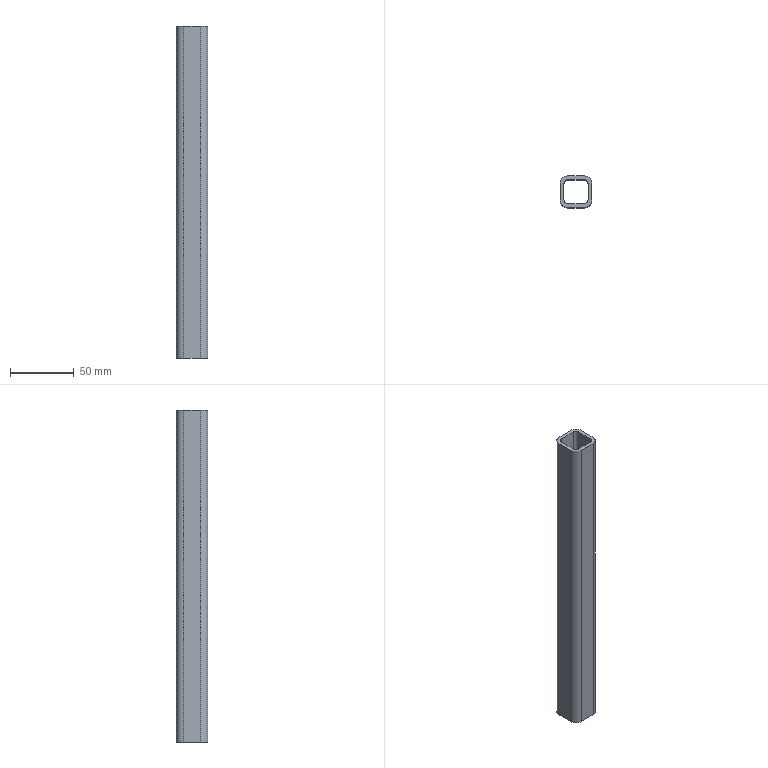Part | STEP file | ISO 10799-2 25x25x3 1784906820679 | 1 solid | 18 faces | box 25 x 25 x 261 mm | volume 62855 mm3 | plane 10 | cylinder 8 | commonest cylinder face diameters 6 x4 12 x4
STEP:
#1=CARTESIAN_POINT('',(-6.5,-9.5,286.));
#2=VERTEX_POINT('',#1);
#3=CARTESIAN_POINT('',(6.5,-9.5,286.));
#4=VERTEX_POINT('',#3);
#5=CARTESIAN_POINT('',(3.25,-9.5,286.));
#6=DIRECTION('',(1.,0.,0.));
#7=VECTOR('',#6,10.);
#8=LINE('',#5,#7);
#9=EDGE_CURVE('',#2,#4,#8,.T.);
#10=ORIENTED_EDGE('',*,*,#9,.T.);
#11=CARTESIAN_POINT('',(6.5,-9.5,25.));
#12=VERTEX_POINT('',#11);
#13=CARTESIAN_POINT('',(6.5,-9.5,0.));
#14=DIRECTION('',(0.,0.,1.));
#15=VECTOR('',#14,10.);
#16=LINE('',#13,#15);
#17=EDGE_CURVE('',#12,#4,#16,.T.);
#18=ORIENTED_EDGE('',*,*,#17,.F.);
#19=CARTESIAN_POINT('',(-6.5,-9.5,25.));
#20=VERTEX_POINT('',#19);
#21=CARTESIAN_POINT('',(3.25,-9.5,25.));
#22=DIRECTION('',(1.,0.,0.));
#23=VECTOR('',#22,10.);
#24=LINE('',#21,#23);
#25=EDGE_CURVE('',#20,#12,#24,.T.);
#26=ORIENTED_EDGE('',*,*,#25,.F.);
#27=CARTESIAN_POINT('',(-6.5,-9.5,0.));
#28=DIRECTION('',(0.,0.,1.));
#29=VECTOR('',#28,10.);
#30=LINE('',#27,#29);
#31=EDGE_CURVE('',#20,#2,#30,.T.);
#32=ORIENTED_EDGE('',*,*,#31,.T.);
#33=EDGE_LOOP('',(#10,#18,#26,#32));
#34=FACE_OUTER_BOUND('',#33,.T.);
#35=CARTESIAN_POINT('',(6.5,-9.5,0.));
#36=DIRECTION('',(0.,-1.,0.));
#37=DIRECTION('',(0.,0.,-1.));
#38=AXIS2_PLACEMENT_3D('',#35,#36,#37);
#39=PLANE('',#38);
#40=ADVANCED_FACE('',(#34),#39,.F.);
#41=CARTESIAN_POINT('',(9.5,-6.5,286.));
#42=VERTEX_POINT('',#41);
#43=CARTESIAN_POINT('',(6.5,-6.5,286.));
#44=DIRECTION('',(0.,0.,1.));
#45=DIRECTION('',(0.,1.,0.));
#46=AXIS2_PLACEMENT_3D('',#43,#44,#45);
#47=CIRCLE('',#46,3.);
#48=EDGE_CURVE('',#4,#42,#47,.T.);
#49=ORIENTED_EDGE('',*,*,#48,.T.);
#50=CARTESIAN_POINT('',(9.5,-6.5,25.));
#51=VERTEX_POINT('',#50);
#52=CARTESIAN_POINT('',(9.5,-6.5,0.));
#53=DIRECTION('',(0.,0.,1.));
#54=VECTOR('',#53,10.);
#55=LINE('',#52,#54);
#56=EDGE_CURVE('',#51,#42,#55,.T.);
#57=ORIENTED_EDGE('',*,*,#56,.F.);
#58=CARTESIAN_POINT('',(6.5,-6.5,25.));
#59=DIRECTION('',(0.,0.,1.));
#60=DIRECTION('',(0.,1.,0.));
#61=AXIS2_PLACEMENT_3D('',#58,#59,#60);
#62=CIRCLE('',#61,3.);
#63=EDGE_CURVE('',#12,#51,#62,.T.);
#64=ORIENTED_EDGE('',*,*,#63,.F.);
#65=ORIENTED_EDGE('',*,*,#17,.T.);
#66=EDGE_LOOP('',(#49,#57,#64,#65));
#67=FACE_OUTER_BOUND('',#66,.T.);
#68=CARTESIAN_POINT('',(6.5,-6.5,0.));
#69=DIRECTION('',(0.,0.,1.));
#70=DIRECTION('',(0.,1.,0.));
#71=AXIS2_PLACEMENT_3D('',#68,#69,#70);
#72=CYLINDRICAL_SURFACE('',#71,3.);
#73=ADVANCED_FACE('',(#67),#72,.F.);
#74=CARTESIAN_POINT('',(9.5,6.5,286.));
#75=VERTEX_POINT('',#74);
#76=CARTESIAN_POINT('',(9.5,3.25,286.));
#77=DIRECTION('',(0.,1.,0.));
#78=VECTOR('',#77,10.);
#79=LINE('',#76,#78);
#80=EDGE_CURVE('',#42,#75,#79,.T.);
#81=ORIENTED_EDGE('',*,*,#80,.T.);
#82=CARTESIAN_POINT('',(9.5,6.5,25.));
#83=VERTEX_POINT('',#82);
#84=CARTESIAN_POINT('',(9.5,6.5,0.));
#85=DIRECTION('',(0.,0.,1.));
#86=VECTOR('',#85,10.);
#87=LINE('',#84,#86);
#88=EDGE_CURVE('',#83,#75,#87,.T.);
#89=ORIENTED_EDGE('',*,*,#88,.F.);
#90=CARTESIAN_POINT('',(9.5,3.25,25.));
#91=DIRECTION('',(0.,1.,0.));
#92=VECTOR('',#91,10.);
#93=LINE('',#90,#92);
#94=EDGE_CURVE('',#51,#83,#93,.T.);
#95=ORIENTED_EDGE('',*,*,#94,.F.);
#96=ORIENTED_EDGE('',*,*,#56,.T.);
#97=EDGE_LOOP('',(#81,#89,#95,#96));
#98=FACE_OUTER_BOUND('',#97,.T.);
#99=CARTESIAN_POINT('',(9.5,6.5,0.));
#100=DIRECTION('',(1.,0.,0.));
#101=DIRECTION('',(0.,0.,-1.));
#102=AXIS2_PLACEMENT_3D('',#99,#100,#101);
#103=PLANE('',#102);
#104=ADVANCED_FACE('',(#98),#103,.F.);
#105=CARTESIAN_POINT('',(6.5,9.5,286.));
#106=VERTEX_POINT('',#105);
#107=CARTESIAN_POINT('',(6.5,6.5,286.));
#108=DIRECTION('',(0.,0.,1.));
#109=DIRECTION('',(-1.,0.,0.));
#110=AXIS2_PLACEMENT_3D('',#107,#108,#109);
#111=CIRCLE('',#110,3.);
#112=EDGE_CURVE('',#75,#106,#111,.T.);
#113=ORIENTED_EDGE('',*,*,#112,.T.);
#114=CARTESIAN_POINT('',(6.5,9.5,25.));
#115=VERTEX_POINT('',#114);
#116=CARTESIAN_POINT('',(6.5,9.5,0.));
#117=DIRECTION('',(0.,0.,1.));
#118=VECTOR('',#117,10.);
#119=LINE('',#116,#118);
#120=EDGE_CURVE('',#115,#106,#119,.T.);
#121=ORIENTED_EDGE('',*,*,#120,.F.);
#122=CARTESIAN_POINT('',(6.5,6.5,25.));
#123=DIRECTION('',(0.,0.,1.));
#124=DIRECTION('',(-1.,0.,0.));
#125=AXIS2_PLACEMENT_3D('',#122,#123,#124);
#126=CIRCLE('',#125,3.);
#127=EDGE_CURVE('',#83,#115,#126,.T.);
#128=ORIENTED_EDGE('',*,*,#127,.F.);
#129=ORIENTED_EDGE('',*,*,#88,.T.);
#130=EDGE_LOOP('',(#113,#121,#128,#129));
#131=FACE_OUTER_BOUND('',#130,.T.);
#132=CARTESIAN_POINT('',(6.5,6.5,0.));
#133=DIRECTION('',(0.,0.,1.));
#134=DIRECTION('',(-1.,0.,0.));
#135=AXIS2_PLACEMENT_3D('',#132,#133,#134);
#136=CYLINDRICAL_SURFACE('',#135,3.);
#137=ADVANCED_FACE('',(#131),#136,.F.);
#138=CARTESIAN_POINT('',(12.5,6.5,286.));
#139=VERTEX_POINT('',#138);
#140=CARTESIAN_POINT('',(12.5,-6.5,286.));
#141=VERTEX_POINT('',#140);
#142=CARTESIAN_POINT('',(12.5,3.25,286.));
#143=DIRECTION('',(0.,-1.,0.));
#144=VECTOR('',#143,10.);
#145=LINE('',#142,#144);
#146=EDGE_CURVE('',#139,#141,#145,.T.);
#147=ORIENTED_EDGE('',*,*,#146,.T.);
#148=CARTESIAN_POINT('',(12.5,-6.5,25.));
#149=VERTEX_POINT('',#148);
#150=CARTESIAN_POINT('',(12.5,-6.5,0.));
#151=DIRECTION('',(0.,0.,1.));
#152=VECTOR('',#151,10.);
#153=LINE('',#150,#152);
#154=EDGE_CURVE('',#149,#141,#153,.T.);
#155=ORIENTED_EDGE('',*,*,#154,.F.);
#156=CARTESIAN_POINT('',(12.5,6.5,25.));
#157=VERTEX_POINT('',#156);
#158=CARTESIAN_POINT('',(12.5,3.25,25.));
#159=DIRECTION('',(0.,-1.,0.));
#160=VECTOR('',#159,10.);
#161=LINE('',#158,#160);
#162=EDGE_CURVE('',#157,#149,#161,.T.);
#163=ORIENTED_EDGE('',*,*,#162,.F.);
#164=CARTESIAN_POINT('',(12.5,6.5,0.));
#165=DIRECTION('',(0.,0.,1.));
#166=VECTOR('',#165,10.);
#167=LINE('',#164,#166);
#168=EDGE_CURVE('',#157,#139,#167,.T.);
#169=ORIENTED_EDGE('',*,*,#168,.T.);
#170=EDGE_LOOP('',(#147,#155,#163,#169));
#171=FACE_OUTER_BOUND('',#170,.T.);
#172=CARTESIAN_POINT('',(12.5,6.5,0.));
#173=DIRECTION('',(1.,0.,0.));
#174=DIRECTION('',(0.,0.,-1.));
#175=AXIS2_PLACEMENT_3D('',#172,#173,#174);
#176=PLANE('',#175);
#177=ADVANCED_FACE('',(#171),#176,.T.);
#178=CARTESIAN_POINT('',(6.5,-12.5,286.));
#179=VERTEX_POINT('',#178);
#180=CARTESIAN_POINT('',(6.5,-6.5,286.));
#181=DIRECTION('',(0.,0.,-1.));
#182=DIRECTION('',(0.,1.,0.));
#183=AXIS2_PLACEMENT_3D('',#180,#181,#182);
#184=CIRCLE('',#183,6.);
#185=EDGE_CURVE('',#141,#179,#184,.T.);
#186=ORIENTED_EDGE('',*,*,#185,.T.);
#187=CARTESIAN_POINT('',(6.5,-12.5,25.));
#188=VERTEX_POINT('',#187);
#189=CARTESIAN_POINT('',(6.5,-12.5,0.));
#190=DIRECTION('',(0.,0.,1.));
#191=VECTOR('',#190,10.);
#192=LINE('',#189,#191);
#193=EDGE_CURVE('',#188,#179,#192,.T.);
#194=ORIENTED_EDGE('',*,*,#193,.F.);
#195=CARTESIAN_POINT('',(6.5,-6.5,25.));
#196=DIRECTION('',(0.,0.,-1.));
#197=DIRECTION('',(0.,1.,0.));
#198=AXIS2_PLACEMENT_3D('',#195,#196,#197);
#199=CIRCLE('',#198,6.);
#200=EDGE_CURVE('',#149,#188,#199,.T.);
#201=ORIENTED_EDGE('',*,*,#200,.F.);
#202=ORIENTED_EDGE('',*,*,#154,.T.);
#203=EDGE_LOOP('',(#186,#194,#201,#202));
#204=FACE_OUTER_BOUND('',#203,.T.);
#205=CARTESIAN_POINT('',(6.5,-6.5,0.));
#206=DIRECTION('',(0.,0.,1.));
#207=DIRECTION('',(0.,1.,0.));
#208=AXIS2_PLACEMENT_3D('',#205,#206,#207);
#209=CYLINDRICAL_SURFACE('',#208,6.);
#210=ADVANCED_FACE('',(#204),#209,.T.);
#211=CARTESIAN_POINT('',(-6.5,-12.5,286.));
#212=VERTEX_POINT('',#211);
#213=CARTESIAN_POINT('',(3.25,-12.5,286.));
#214=DIRECTION('',(-1.,0.,0.));
#215=VECTOR('',#214,10.);
#216=LINE('',#213,#215);
#217=EDGE_CURVE('',#179,#212,#216,.T.);
#218=ORIENTED_EDGE('',*,*,#217,.T.);
#219=CARTESIAN_POINT('',(-6.5,-12.5,25.));
#220=VERTEX_POINT('',#219);
#221=CARTESIAN_POINT('',(-6.5,-12.5,0.));
#222=DIRECTION('',(0.,0.,1.));
#223=VECTOR('',#222,10.);
#224=LINE('',#221,#223);
#225=EDGE_CURVE('',#220,#212,#224,.T.);
#226=ORIENTED_EDGE('',*,*,#225,.F.);
#227=CARTESIAN_POINT('',(3.25,-12.5,25.));
#228=DIRECTION('',(-1.,0.,0.));
#229=VECTOR('',#228,10.);
#230=LINE('',#227,#229);
#231=EDGE_CURVE('',#188,#220,#230,.T.);
#232=ORIENTED_EDGE('',*,*,#231,.F.);
#233=ORIENTED_EDGE('',*,*,#193,.T.);
#234=EDGE_LOOP('',(#218,#226,#232,#233));
#235=FACE_OUTER_BOUND('',#234,.T.);
#236=CARTESIAN_POINT('',(6.5,-12.5,0.));
#237=DIRECTION('',(0.,-1.,0.));
#238=DIRECTION('',(0.,0.,-1.));
#239=AXIS2_PLACEMENT_3D('',#236,#237,#238);
#240=PLANE('',#239);
#241=ADVANCED_FACE('',(#235),#240,.T.);
#242=CARTESIAN_POINT('',(-12.5,-6.5,286.));
#243=VERTEX_POINT('',#242);
#244=CARTESIAN_POINT('',(-6.5,-6.5,286.));
#245=DIRECTION('',(0.,0.,-1.));
#246=DIRECTION('',(1.,0.,0.));
#247=AXIS2_PLACEMENT_3D('',#244,#245,#246);
#248=CIRCLE('',#247,6.);
#249=EDGE_CURVE('',#212,#243,#248,.T.);
#250=ORIENTED_EDGE('',*,*,#249,.T.);
#251=CARTESIAN_POINT('',(-12.5,-6.5,25.));
#252=VERTEX_POINT('',#251);
#253=CARTESIAN_POINT('',(-12.5,-6.5,0.));
#254=DIRECTION('',(0.,0.,1.));
#255=VECTOR('',#254,10.);
#256=LINE('',#253,#255);
#257=EDGE_CURVE('',#252,#243,#256,.T.);
#258=ORIENTED_EDGE('',*,*,#257,.F.);
#259=CARTESIAN_POINT('',(-6.5,-6.5,25.));
#260=DIRECTION('',(0.,0.,-1.));
#261=DIRECTION('',(1.,0.,0.));
#262=AXIS2_PLACEMENT_3D('',#259,#260,#261);
#263=CIRCLE('',#262,6.);
#264=EDGE_CURVE('',#220,#252,#263,.T.);
#265=ORIENTED_EDGE('',*,*,#264,.F.);
#266=ORIENTED_EDGE('',*,*,#225,.T.);
#267=EDGE_LOOP('',(#250,#258,#265,#266));
#268=FACE_OUTER_BOUND('',#267,.T.);
#269=CARTESIAN_POINT('',(-6.5,-6.5,0.));
#270=DIRECTION('',(0.,0.,1.));
#271=DIRECTION('',(1.,0.,0.));
#272=AXIS2_PLACEMENT_3D('',#269,#270,#271);
#273=CYLINDRICAL_SURFACE('',#272,6.);
#274=ADVANCED_FACE('',(#268),#273,.T.);
#275=CARTESIAN_POINT('',(-6.5,9.5,286.));
#276=VERTEX_POINT('',#275);
#277=CARTESIAN_POINT('',(-3.25,9.5,286.));
#278=DIRECTION('',(-1.,0.,0.));
#279=VECTOR('',#278,10.);
#280=LINE('',#277,#279);
#281=EDGE_CURVE('',#106,#276,#280,.T.);
#282=ORIENTED_EDGE('',*,*,#281,.T.);
#283=CARTESIAN_POINT('',(-6.5,9.5,25.));
#284=VERTEX_POINT('',#283);
#285=CARTESIAN_POINT('',(-6.5,9.5,0.));
#286=DIRECTION('',(0.,0.,1.));
#287=VECTOR('',#286,10.);
#288=LINE('',#285,#287);
#289=EDGE_CURVE('',#284,#276,#288,.T.);
#290=ORIENTED_EDGE('',*,*,#289,.F.);
#291=CARTESIAN_POINT('',(-3.25,9.5,25.));
#292=DIRECTION('',(-1.,0.,0.));
#293=VECTOR('',#292,10.);
#294=LINE('',#291,#293);
#295=EDGE_CURVE('',#115,#284,#294,.T.);
#296=ORIENTED_EDGE('',*,*,#295,.F.);
#297=ORIENTED_EDGE('',*,*,#120,.T.);
#298=EDGE_LOOP('',(#282,#290,#296,#297));
#299=FACE_OUTER_BOUND('',#298,.T.);
#300=CARTESIAN_POINT('',(-6.5,9.5,0.));
#301=DIRECTION('',(0.,1.,0.));
#302=DIRECTION('',(0.,0.,1.));
#303=AXIS2_PLACEMENT_3D('',#300,#301,#302);
#304=PLANE('',#303);
#305=ADVANCED_FACE('',(#299),#304,.F.);
#306=CARTESIAN_POINT('',(-9.5,-6.5,286.));
#307=VERTEX_POINT('',#306);
#308=CARTESIAN_POINT('',(-6.5,-6.5,286.));
#309=DIRECTION('',(0.,0.,1.));
#310=DIRECTION('',(1.,0.,0.));
#311=AXIS2_PLACEMENT_3D('',#308,#309,#310);
#312=CIRCLE('',#311,3.);
#313=EDGE_CURVE('',#307,#2,#312,.T.);
#314=ORIENTED_EDGE('',*,*,#313,.T.);
#315=ORIENTED_EDGE('',*,*,#31,.F.);
#316=CARTESIAN_POINT('',(-9.5,-6.5,25.));
#317=VERTEX_POINT('',#316);
#318=CARTESIAN_POINT('',(-6.5,-6.5,25.));
#319=DIRECTION('',(0.,0.,1.));
#320=DIRECTION('',(1.,0.,0.));
#321=AXIS2_PLACEMENT_3D('',#318,#319,#320);
#322=CIRCLE('',#321,3.);
#323=EDGE_CURVE('',#317,#20,#322,.T.);
#324=ORIENTED_EDGE('',*,*,#323,.F.);
#325=CARTESIAN_POINT('',(-9.5,-6.5,0.));
#326=DIRECTION('',(0.,0.,1.));
#327=VECTOR('',#326,10.);
#328=LINE('',#325,#327);
#329=EDGE_CURVE('',#317,#307,#328,.T.);
#330=ORIENTED_EDGE('',*,*,#329,.T.);
#331=EDGE_LOOP('',(#314,#315,#324,#330));
#332=FACE_OUTER_BOUND('',#331,.T.);
#333=CARTESIAN_POINT('',(-6.5,-6.5,0.));
#334=DIRECTION('',(0.,0.,1.));
#335=DIRECTION('',(1.,0.,0.));
#336=AXIS2_PLACEMENT_3D('',#333,#334,#335);
#337=CYLINDRICAL_SURFACE('',#336,3.);
#338=ADVANCED_FACE('',(#332),#337,.F.);
#339=CARTESIAN_POINT('',(-9.5,6.5,286.));
#340=VERTEX_POINT('',#339);
#341=CARTESIAN_POINT('',(-9.5,-3.25,286.));
#342=DIRECTION('',(0.,-1.,0.));
#343=VECTOR('',#342,10.);
#344=LINE('',#341,#343);
#345=EDGE_CURVE('',#340,#307,#344,.T.);
#346=ORIENTED_EDGE('',*,*,#345,.T.);
#347=ORIENTED_EDGE('',*,*,#329,.F.);
#348=CARTESIAN_POINT('',(-9.5,6.5,25.));
#349=VERTEX_POINT('',#348);
#350=CARTESIAN_POINT('',(-9.5,-3.25,25.));
#351=DIRECTION('',(0.,-1.,0.));
#352=VECTOR('',#351,10.);
#353=LINE('',#350,#352);
#354=EDGE_CURVE('',#349,#317,#353,.T.);
#355=ORIENTED_EDGE('',*,*,#354,.F.);
#356=CARTESIAN_POINT('',(-9.5,6.5,0.));
#357=DIRECTION('',(0.,0.,1.));
#358=VECTOR('',#357,10.);
#359=LINE('',#356,#358);
#360=EDGE_CURVE('',#349,#340,#359,.T.);
#361=ORIENTED_EDGE('',*,*,#360,.T.);
#362=EDGE_LOOP('',(#346,#347,#355,#361));
#363=FACE_OUTER_BOUND('',#362,.T.);
#364=CARTESIAN_POINT('',(-9.5,-6.5,0.));
#365=DIRECTION('',(-1.,0.,0.));
#366=DIRECTION('',(0.,0.,1.));
#367=AXIS2_PLACEMENT_3D('',#364,#365,#366);
#368=PLANE('',#367);
#369=ADVANCED_FACE('',(#363),#368,.F.);
#370=CARTESIAN_POINT('',(-6.5,6.5,286.));
#371=DIRECTION('',(0.,0.,1.));
#372=DIRECTION('',(0.,-1.,0.));
#373=AXIS2_PLACEMENT_3D('',#370,#371,#372);
#374=CIRCLE('',#373,3.);
#375=EDGE_CURVE('',#276,#340,#374,.T.);
#376=ORIENTED_EDGE('',*,*,#375,.T.);
#377=ORIENTED_EDGE('',*,*,#360,.F.);
#378=CARTESIAN_POINT('',(-6.5,6.5,25.));
#379=DIRECTION('',(0.,0.,1.));
#380=DIRECTION('',(0.,-1.,0.));
#381=AXIS2_PLACEMENT_3D('',#378,#379,#380);
#382=CIRCLE('',#381,3.);
#383=EDGE_CURVE('',#284,#349,#382,.T.);
#384=ORIENTED_EDGE('',*,*,#383,.F.);
#385=ORIENTED_EDGE('',*,*,#289,.T.);
#386=EDGE_LOOP('',(#376,#377,#384,#385));
#387=FACE_OUTER_BOUND('',#386,.T.);
#388=CARTESIAN_POINT('',(-6.5,6.5,0.));
#389=DIRECTION('',(0.,0.,1.));
#390=DIRECTION('',(0.,-1.,0.));
#391=AXIS2_PLACEMENT_3D('',#388,#389,#390);
#392=CYLINDRICAL_SURFACE('',#391,3.);
#393=ADVANCED_FACE('',(#387),#392,.F.);
#394=CARTESIAN_POINT('',(-12.5,6.5,286.));
#395=VERTEX_POINT('',#394);
#396=CARTESIAN_POINT('',(-12.5,-3.25,286.));
#397=DIRECTION('',(0.,1.,0.));
#398=VECTOR('',#397,10.);
#399=LINE('',#396,#398);
#400=EDGE_CURVE('',#243,#395,#399,.T.);
#401=ORIENTED_EDGE('',*,*,#400,.T.);
#402=CARTESIAN_POINT('',(-12.5,6.5,25.));
#403=VERTEX_POINT('',#402);
#404=CARTESIAN_POINT('',(-12.5,6.5,0.));
#405=DIRECTION('',(0.,0.,1.));
#406=VECTOR('',#405,10.);
#407=LINE('',#404,#406);
#408=EDGE_CURVE('',#403,#395,#407,.T.);
#409=ORIENTED_EDGE('',*,*,#408,.F.);
#410=CARTESIAN_POINT('',(-12.5,-3.25,25.));
#411=DIRECTION('',(0.,1.,0.));
#412=VECTOR('',#411,10.);
#413=LINE('',#410,#412);
#414=EDGE_CURVE('',#252,#403,#413,.T.);
#415=ORIENTED_EDGE('',*,*,#414,.F.);
#416=ORIENTED_EDGE('',*,*,#257,.T.);
#417=EDGE_LOOP('',(#401,#409,#415,#416));
#418=FACE_OUTER_BOUND('',#417,.T.);
#419=CARTESIAN_POINT('',(-12.5,-6.5,0.));
#420=DIRECTION('',(-1.,0.,0.));
#421=DIRECTION('',(0.,0.,1.));
#422=AXIS2_PLACEMENT_3D('',#419,#420,#421);
#423=PLANE('',#422);
#424=ADVANCED_FACE('',(#418),#423,.T.);
#425=CARTESIAN_POINT('',(-6.5,12.5,286.));
#426=VERTEX_POINT('',#425);
#427=CARTESIAN_POINT('',(-6.5,6.5,286.));
#428=DIRECTION('',(0.,0.,-1.));
#429=DIRECTION('',(0.,-1.,0.));
#430=AXIS2_PLACEMENT_3D('',#427,#428,#429);
#431=CIRCLE('',#430,6.);
#432=EDGE_CURVE('',#395,#426,#431,.T.);
#433=ORIENTED_EDGE('',*,*,#432,.T.);
#434=CARTESIAN_POINT('',(-6.5,12.5,25.));
#435=VERTEX_POINT('',#434);
#436=CARTESIAN_POINT('',(-6.5,12.5,0.));
#437=DIRECTION('',(0.,0.,1.));
#438=VECTOR('',#437,10.);
#439=LINE('',#436,#438);
#440=EDGE_CURVE('',#435,#426,#439,.T.);
#441=ORIENTED_EDGE('',*,*,#440,.F.);
#442=CARTESIAN_POINT('',(-6.5,6.5,25.));
#443=DIRECTION('',(0.,0.,-1.));
#444=DIRECTION('',(0.,-1.,0.));
#445=AXIS2_PLACEMENT_3D('',#442,#443,#444);
#446=CIRCLE('',#445,6.);
#447=EDGE_CURVE('',#403,#435,#446,.T.);
#448=ORIENTED_EDGE('',*,*,#447,.F.);
#449=ORIENTED_EDGE('',*,*,#408,.T.);
#450=EDGE_LOOP('',(#433,#441,#448,#449));
#451=FACE_OUTER_BOUND('',#450,.T.);
#452=CARTESIAN_POINT('',(-6.5,6.5,0.));
#453=DIRECTION('',(0.,0.,1.));
#454=DIRECTION('',(0.,-1.,0.));
#455=AXIS2_PLACEMENT_3D('',#452,#453,#454);
#456=CYLINDRICAL_SURFACE('',#455,6.);
#457=ADVANCED_FACE('',(#451),#456,.T.);
#458=CARTESIAN_POINT('',(6.5,12.5,286.));
#459=VERTEX_POINT('',#458);
#460=CARTESIAN_POINT('',(-3.25,12.5,286.));
#461=DIRECTION('',(1.,0.,0.));
#462=VECTOR('',#461,10.);
#463=LINE('',#460,#462);
#464=EDGE_CURVE('',#426,#459,#463,.T.);
#465=ORIENTED_EDGE('',*,*,#464,.T.);
#466=CARTESIAN_POINT('',(6.5,12.5,25.));
#467=VERTEX_POINT('',#466);
#468=CARTESIAN_POINT('',(6.5,12.5,0.));
#469=DIRECTION('',(0.,0.,1.));
#470=VECTOR('',#469,10.);
#471=LINE('',#468,#470);
#472=EDGE_CURVE('',#467,#459,#471,.T.);
#473=ORIENTED_EDGE('',*,*,#472,.F.);
#474=CARTESIAN_POINT('',(-3.25,12.5,25.));
#475=DIRECTION('',(1.,0.,0.));
#476=VECTOR('',#475,10.);
#477=LINE('',#474,#476);
#478=EDGE_CURVE('',#435,#467,#477,.T.);
#479=ORIENTED_EDGE('',*,*,#478,.F.);
#480=ORIENTED_EDGE('',*,*,#440,.T.);
#481=EDGE_LOOP('',(#465,#473,#479,#480));
#482=FACE_OUTER_BOUND('',#481,.T.);
#483=CARTESIAN_POINT('',(-6.5,12.5,0.));
#484=DIRECTION('',(0.,1.,0.));
#485=DIRECTION('',(0.,0.,1.));
#486=AXIS2_PLACEMENT_3D('',#483,#484,#485);
#487=PLANE('',#486);
#488=ADVANCED_FACE('',(#482),#487,.T.);
#489=CARTESIAN_POINT('',(6.5,6.5,286.));
#490=DIRECTION('',(0.,0.,-1.));
#491=DIRECTION('',(-1.,0.,0.));
#492=AXIS2_PLACEMENT_3D('',#489,#490,#491);
#493=CIRCLE('',#492,6.);
#494=EDGE_CURVE('',#459,#139,#493,.T.);
#495=ORIENTED_EDGE('',*,*,#494,.T.);
#496=ORIENTED_EDGE('',*,*,#168,.F.);
#497=CARTESIAN_POINT('',(6.5,6.5,25.));
#498=DIRECTION('',(0.,0.,-1.));
#499=DIRECTION('',(-1.,0.,0.));
#500=AXIS2_PLACEMENT_3D('',#497,#498,#499);
#501=CIRCLE('',#500,6.);
#502=EDGE_CURVE('',#467,#157,#501,.T.);
#503=ORIENTED_EDGE('',*,*,#502,.F.);
#504=ORIENTED_EDGE('',*,*,#472,.T.);
#505=EDGE_LOOP('',(#495,#496,#503,#504));
#506=FACE_OUTER_BOUND('',#505,.T.);
#507=CARTESIAN_POINT('',(6.5,6.5,0.));
#508=DIRECTION('',(0.,0.,1.));
#509=DIRECTION('',(-1.,0.,0.));
#510=AXIS2_PLACEMENT_3D('',#507,#508,#509);
#511=CYLINDRICAL_SURFACE('',#510,6.);
#512=ADVANCED_FACE('',(#506),#511,.T.);
#513=ORIENTED_EDGE('',*,*,#414,.T.);
#514=ORIENTED_EDGE('',*,*,#447,.T.);
#515=ORIENTED_EDGE('',*,*,#478,.T.);
#516=ORIENTED_EDGE('',*,*,#502,.T.);
#517=ORIENTED_EDGE('',*,*,#162,.T.);
#518=ORIENTED_EDGE('',*,*,#200,.T.);
#519=ORIENTED_EDGE('',*,*,#231,.T.);
#520=ORIENTED_EDGE('',*,*,#264,.T.);
#521=EDGE_LOOP('',(#513,#514,#515,#516,#517,#518,#519,#520));
#522=FACE_OUTER_BOUND('',#521,.T.);
#523=ORIENTED_EDGE('',*,*,#295,.T.);
#524=ORIENTED_EDGE('',*,*,#383,.T.);
#525=ORIENTED_EDGE('',*,*,#354,.T.);
#526=ORIENTED_EDGE('',*,*,#323,.T.);
#527=ORIENTED_EDGE('',*,*,#25,.T.);
#528=ORIENTED_EDGE('',*,*,#63,.T.);
#529=ORIENTED_EDGE('',*,*,#94,.T.);
#530=ORIENTED_EDGE('',*,*,#127,.T.);
#531=EDGE_LOOP('',(#523,#524,#525,#526,#527,#528,#529,#530));
#532=FACE_BOUND('',#531,.T.);
#533=CARTESIAN_POINT('',(0.,0.,25.));
#534=DIRECTION('',(0.,0.,1.));
#535=DIRECTION('',(1.,0.,0.));
#536=AXIS2_PLACEMENT_3D('',#533,#534,#535);
#537=PLANE('',#536);
#538=ADVANCED_FACE('',(#522,#532),#537,.F.);
#539=ORIENTED_EDGE('',*,*,#400,.F.);
#540=ORIENTED_EDGE('',*,*,#249,.F.);
#541=ORIENTED_EDGE('',*,*,#217,.F.);
#542=ORIENTED_EDGE('',*,*,#185,.F.);
#543=ORIENTED_EDGE('',*,*,#146,.F.);
#544=ORIENTED_EDGE('',*,*,#494,.F.);
#545=ORIENTED_EDGE('',*,*,#464,.F.);
#546=ORIENTED_EDGE('',*,*,#432,.F.);
#547=EDGE_LOOP('',(#539,#540,#541,#542,#543,#544,#545,#546));
#548=FACE_OUTER_BOUND('',#547,.T.);
#549=ORIENTED_EDGE('',*,*,#281,.F.);
#550=ORIENTED_EDGE('',*,*,#112,.F.);
#551=ORIENTED_EDGE('',*,*,#80,.F.);
#552=ORIENTED_EDGE('',*,*,#48,.F.);
#553=ORIENTED_EDGE('',*,*,#9,.F.);
#554=ORIENTED_EDGE('',*,*,#313,.F.);
#555=ORIENTED_EDGE('',*,*,#345,.F.);
#556=ORIENTED_EDGE('',*,*,#375,.F.);
#557=EDGE_LOOP('',(#549,#550,#551,#552,#553,#554,#555,#556));
#558=FACE_BOUND('',#557,.T.);
#559=CARTESIAN_POINT('',(0.,0.,286.));
#560=DIRECTION('',(0.,0.,1.));
#561=DIRECTION('',(1.,0.,0.));
#562=AXIS2_PLACEMENT_3D('',#559,#560,#561);
#563=PLANE('',#562);
#564=ADVANCED_FACE('',(#548,#558),#563,.T.);
#565=CLOSED_SHELL('',(#40,#73,#104,#137,#177,#210,#241,#274,#305,#338,#369,#393,#424,#457,#488,#512,#538,#564));
#566=MANIFOLD_SOLID_BREP('',#565);
#567=(LENGTH_UNIT()NAMED_UNIT(*)SI_UNIT(.MILLI.,.METRE.));
#568=UNCERTAINTY_MEASURE_WITH_UNIT(LENGTH_MEASURE(0.01),#567,'','');
#569=(NAMED_UNIT(*)PLANE_ANGLE_UNIT()SI_UNIT($,.RADIAN.));
#570=(NAMED_UNIT(*)SI_UNIT($,.STERADIAN.)SOLID_ANGLE_UNIT());
#571=(GEOMETRIC_REPRESENTATION_CONTEXT(3)GLOBAL_UNCERTAINTY_ASSIGNED_CONTEXT((#568))GLOBAL_UNIT_ASSIGNED_CONTEXT((#567,#569,#570))REPRESENTATION_CONTEXT('',''));
#572=ADVANCED_BREP_SHAPE_REPRESENTATION('',(#566),#571);